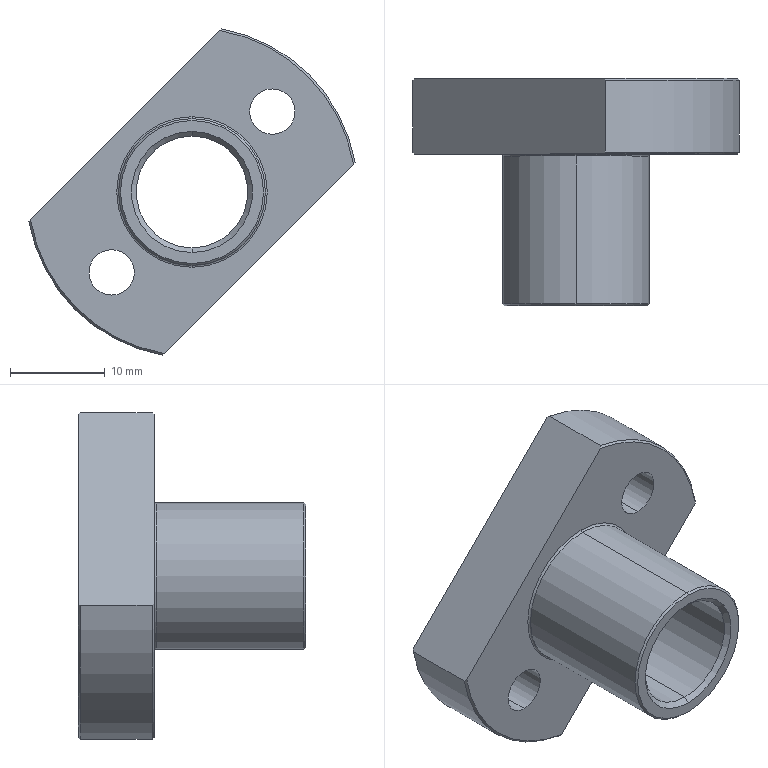Part | SolidWorks | features 3DProfileFeature 2, Chamfer 2, HoleWzd 2, Fillet 1, ICE 1, Revolution 1 | 1 solid | 33 faces | box 34.452 x 24 x 34.452 mm | volume 5075 mm3 | cylinder 14 | cone 10 | plane 7 | torus 2 | commonest cylinder face diameters 4.8 x4 8 x4 11.8 x2 15.5 x2 35 x2
STEP:
#1=CARTESIAN_POINT('',(0.,0.5,5.9));
#2=VERTEX_POINT('',#1);
#3=CARTESIAN_POINT('',(0.,0.5,-5.9));
#4=VERTEX_POINT('',#3);
#5=CARTESIAN_POINT('',(0.,0.5,0.));
#6=DIRECTION('',(0.,-1.,0.));
#7=DIRECTION('',(0.,0.,1.));
#8=AXIS2_PLACEMENT_3D('',#5,#6,#7);
#9=CIRCLE('',#8,5.9);
#10=EDGE_CURVE('',#2,#4,#9,.T.);
#11=ORIENTED_EDGE('',*,*,#10,.F.);
#12=CARTESIAN_POINT('',(0.,0.,6.4));
#13=VERTEX_POINT('',#12);
#14=CARTESIAN_POINT('',(0.,0.,6.4));
#15=DIRECTION('',(0.,-0.7071,0.7071));
#16=VECTOR('',#15,1000.);
#17=LINE('',#14,#16);
#18=EDGE_CURVE('',#2,#13,#17,.T.);
#19=ORIENTED_EDGE('',*,*,#18,.T.);
#20=CARTESIAN_POINT('',(0.,0.,-6.4));
#21=VERTEX_POINT('',#20);
#22=CARTESIAN_POINT('',(0.,0.,0.));
#23=DIRECTION('',(0.,1.,0.));
#24=DIRECTION('',(0.,0.,1.));
#25=AXIS2_PLACEMENT_3D('',#22,#23,#24);
#26=CIRCLE('',#25,6.4);
#27=EDGE_CURVE('',#21,#13,#26,.T.);
#28=ORIENTED_EDGE('',*,*,#27,.F.);
#29=CARTESIAN_POINT('',(0.,0.,-6.4));
#30=DIRECTION('',(0.,-0.7071,-0.7071));
#31=VECTOR('',#30,1000.);
#32=LINE('',#29,#31);
#33=EDGE_CURVE('',#4,#21,#32,.T.);
#34=ORIENTED_EDGE('',*,*,#33,.F.);
#35=EDGE_LOOP('',(#11,#19,#28,#34));
#36=FACE_OUTER_BOUND('',#35,.T.);
#37=CARTESIAN_POINT('',(0.,0.,0.));
#38=DIRECTION('',(0.,-1.,0.));
#39=DIRECTION('',(0.,0.,-1.));
#40=AXIS2_PLACEMENT_3D('',#37,#38,#39);
#41=CONICAL_SURFACE('',#40,6.4,0.7854);
#42=ADVANCED_FACE('',(#36),#41,.F.);
#43=CARTESIAN_POINT('',(0.,23.5,-5.9));
#44=VERTEX_POINT('',#43);
#45=CARTESIAN_POINT('',(0.,23.5,5.9));
#46=VERTEX_POINT('',#45);
#47=CARTESIAN_POINT('',(0.,23.5,0.));
#48=DIRECTION('',(0.,1.,0.));
#49=DIRECTION('',(0.,0.,-1.));
#50=AXIS2_PLACEMENT_3D('',#47,#48,#49);
#51=CIRCLE('',#50,5.9);
#52=EDGE_CURVE('',#44,#46,#51,.T.);
#53=ORIENTED_EDGE('',*,*,#52,.F.);
#54=CARTESIAN_POINT('',(0.,24.,-6.4));
#55=VERTEX_POINT('',#54);
#56=CARTESIAN_POINT('',(0.,23.5,-5.9));
#57=DIRECTION('',(0.,0.7071,-0.7071));
#58=VECTOR('',#57,1000.);
#59=LINE('',#56,#58);
#60=EDGE_CURVE('',#44,#55,#59,.T.);
#61=ORIENTED_EDGE('',*,*,#60,.T.);
#62=CARTESIAN_POINT('',(0.,24.,6.4));
#63=VERTEX_POINT('',#62);
#64=CARTESIAN_POINT('',(0.,24.,0.));
#65=DIRECTION('',(0.,-1.,0.));
#66=DIRECTION('',(0.,0.,-1.));
#67=AXIS2_PLACEMENT_3D('',#64,#65,#66);
#68=CIRCLE('',#67,6.4);
#69=EDGE_CURVE('',#63,#55,#68,.T.);
#70=ORIENTED_EDGE('',*,*,#69,.F.);
#71=CARTESIAN_POINT('',(0.,23.5,5.9));
#72=DIRECTION('',(0.,0.7071,0.7071));
#73=VECTOR('',#72,1000.);
#74=LINE('',#71,#73);
#75=EDGE_CURVE('',#46,#63,#74,.T.);
#76=ORIENTED_EDGE('',*,*,#75,.F.);
#77=EDGE_LOOP('',(#53,#61,#70,#76));
#78=FACE_OUTER_BOUND('',#77,.T.);
#79=CARTESIAN_POINT('',(0.,23.5,0.));
#80=DIRECTION('',(0.,1.,0.));
#81=DIRECTION('',(0.,0.,1.));
#82=AXIS2_PLACEMENT_3D('',#79,#80,#81);
#83=CONICAL_SURFACE('',#82,5.9,0.7854);
#84=ADVANCED_FACE('',(#78),#83,.F.);
#85=CARTESIAN_POINT('',(0.,0.,-7.55));
#86=VERTEX_POINT('',#85);
#87=CARTESIAN_POINT('',(0.,0.,7.55));
#88=VERTEX_POINT('',#87);
#89=CARTESIAN_POINT('',(0.,0.,0.));
#90=DIRECTION('',(0.,-1.,0.));
#91=DIRECTION('',(0.,0.,1.));
#92=AXIS2_PLACEMENT_3D('',#89,#90,#91);
#93=CIRCLE('',#92,7.55);
#94=EDGE_CURVE('',#86,#88,#93,.T.);
#95=ORIENTED_EDGE('',*,*,#94,.F.);
#96=CARTESIAN_POINT('',(0.,0.2,-7.75));
#97=VERTEX_POINT('',#96);
#98=CARTESIAN_POINT('',(0.,0.,-7.55));
#99=DIRECTION('',(0.,0.7071,-0.7071));
#100=VECTOR('',#99,1000.);
#101=LINE('',#98,#100);
#102=EDGE_CURVE('',#86,#97,#101,.T.);
#103=ORIENTED_EDGE('',*,*,#102,.T.);
#104=CARTESIAN_POINT('',(0.,0.2,7.75));
#105=VERTEX_POINT('',#104);
#106=CARTESIAN_POINT('',(0.,0.2,0.));
#107=DIRECTION('',(0.,1.,0.));
#108=DIRECTION('',(0.,0.,1.));
#109=AXIS2_PLACEMENT_3D('',#106,#107,#108);
#110=CIRCLE('',#109,7.75);
#111=EDGE_CURVE('',#105,#97,#110,.T.);
#112=ORIENTED_EDGE('',*,*,#111,.F.);
#113=CARTESIAN_POINT('',(0.,0.,7.55));
#114=DIRECTION('',(0.,0.7071,0.7071));
#115=VECTOR('',#114,1000.);
#116=LINE('',#113,#115);
#117=EDGE_CURVE('',#88,#105,#116,.T.);
#118=ORIENTED_EDGE('',*,*,#117,.F.);
#119=EDGE_LOOP('',(#95,#103,#112,#118));
#120=FACE_OUTER_BOUND('',#119,.T.);
#121=CARTESIAN_POINT('',(0.,0.,0.));
#122=DIRECTION('',(0.,1.,0.));
#123=DIRECTION('',(0.,0.,1.));
#124=AXIS2_PLACEMENT_3D('',#121,#122,#123);
#125=CONICAL_SURFACE('',#124,7.55,0.7854);
#126=ADVANCED_FACE('',(#120),#125,.T.);
#127=CARTESIAN_POINT('',(0.,16.,-7.95));
#128=VERTEX_POINT('',#127);
#129=CARTESIAN_POINT('',(0.,16.,7.95));
#130=VERTEX_POINT('',#129);
#131=CARTESIAN_POINT('',(0.,16.,0.));
#132=DIRECTION('',(0.,1.,0.));
#133=DIRECTION('',(0.,0.,1.));
#134=AXIS2_PLACEMENT_3D('',#131,#132,#133);
#135=CIRCLE('',#134,7.95);
#136=EDGE_CURVE('',#128,#130,#135,.T.);
#137=ORIENTED_EDGE('',*,*,#136,.F.);
#138=CARTESIAN_POINT('',(0.,15.8,-7.75));
#139=VERTEX_POINT('',#138);
#140=CARTESIAN_POINT('',(0.,15.8,-7.95));
#141=DIRECTION('',(1.,0.,0.));
#142=DIRECTION('',(0.,0.,-1.));
#143=AXIS2_PLACEMENT_3D('',#140,#141,#142);
#144=CIRCLE('',#143,0.2);
#145=EDGE_CURVE('',#128,#139,#144,.T.);
#146=ORIENTED_EDGE('',*,*,#145,.T.);
#147=CARTESIAN_POINT('',(0.,15.8,7.75));
#148=VERTEX_POINT('',#147);
#149=CARTESIAN_POINT('',(0.,15.8,0.));
#150=DIRECTION('',(0.,-1.,0.));
#151=DIRECTION('',(0.,0.,1.));
#152=AXIS2_PLACEMENT_3D('',#149,#150,#151);
#153=CIRCLE('',#152,7.75);
#154=EDGE_CURVE('',#148,#139,#153,.T.);
#155=ORIENTED_EDGE('',*,*,#154,.F.);
#156=CARTESIAN_POINT('',(0.,15.8,7.95));
#157=DIRECTION('',(-1.,0.,0.));
#158=DIRECTION('',(0.,-1.,0.));
#159=AXIS2_PLACEMENT_3D('',#156,#157,#158);
#160=CIRCLE('',#159,0.2);
#161=EDGE_CURVE('',#130,#148,#160,.T.);
#162=ORIENTED_EDGE('',*,*,#161,.F.);
#163=EDGE_LOOP('',(#137,#146,#155,#162));
#164=FACE_OUTER_BOUND('',#163,.T.);
#165=CARTESIAN_POINT('',(0.,15.8,0.));
#166=DIRECTION('',(0.,1.,0.));
#167=DIRECTION('',(0.,0.,1.));
#168=AXIS2_PLACEMENT_3D('',#165,#166,#167);
#169=TOROIDAL_SURFACE('',#168,7.95,0.2);
#170=ADVANCED_FACE('',(#164),#169,.F.);
#171=CARTESIAN_POINT('',(-8.485,19.4,-12.485));
#172=VERTEX_POINT('',#171);
#173=CARTESIAN_POINT('',(-8.485,19.4,-4.485));
#174=VERTEX_POINT('',#173);
#175=CARTESIAN_POINT('',(-8.485,19.4,-8.485));
#176=DIRECTION('',(0.,1.,0.));
#177=DIRECTION('',(0.,0.,1.));
#178=AXIS2_PLACEMENT_3D('',#175,#176,#177);
#179=CIRCLE('',#178,4.);
#180=EDGE_CURVE('',#172,#174,#179,.T.);
#181=ORIENTED_EDGE('',*,*,#180,.F.);
#182=CARTESIAN_POINT('',(-8.485,24.,-12.485));
#183=VERTEX_POINT('',#182);
#184=CARTESIAN_POINT('',(-8.485,24.,-12.485));
#185=DIRECTION('',(0.,1.,0.));
#186=VECTOR('',#185,1000.);
#187=LINE('',#184,#186);
#188=EDGE_CURVE('',#172,#183,#187,.T.);
#189=ORIENTED_EDGE('',*,*,#188,.T.);
#190=CARTESIAN_POINT('',(-8.485,24.,-4.485));
#191=VERTEX_POINT('',#190);
#192=CARTESIAN_POINT('',(-8.485,24.,-8.485));
#193=DIRECTION('',(0.,1.,0.));
#194=DIRECTION('',(0.,0.,1.));
#195=AXIS2_PLACEMENT_3D('',#192,#193,#194);
#196=CIRCLE('',#195,4.);
#197=EDGE_CURVE('',#183,#191,#196,.T.);
#198=ORIENTED_EDGE('',*,*,#197,.T.);
#199=CARTESIAN_POINT('',(-8.485,24.,-4.485));
#200=DIRECTION('',(0.,1.,0.));
#201=VECTOR('',#200,1000.);
#202=LINE('',#199,#201);
#203=EDGE_CURVE('',#174,#191,#202,.T.);
#204=ORIENTED_EDGE('',*,*,#203,.F.);
#205=EDGE_LOOP('',(#181,#189,#198,#204));
#206=FACE_OUTER_BOUND('',#205,.T.);
#207=CARTESIAN_POINT('',(-8.485,24.,-8.485));
#208=DIRECTION('',(0.,1.,0.));
#209=DIRECTION('',(0.,0.,1.));
#210=AXIS2_PLACEMENT_3D('',#207,#208,#209);
#211=CYLINDRICAL_SURFACE('',#210,4.);
#212=ADVANCED_FACE('',(#206),#211,.F.);
#213=CARTESIAN_POINT('',(-8.485,16.,-10.885));
#214=VERTEX_POINT('',#213);
#215=CARTESIAN_POINT('',(-8.485,16.,-6.085));
#216=VERTEX_POINT('',#215);
#217=CARTESIAN_POINT('',(-8.485,16.,-8.485));
#218=DIRECTION('',(0.,1.,0.));
#219=DIRECTION('',(0.,0.,1.));
#220=AXIS2_PLACEMENT_3D('',#217,#218,#219);
#221=CIRCLE('',#220,2.4);
#222=EDGE_CURVE('',#214,#216,#221,.T.);
#223=ORIENTED_EDGE('',*,*,#222,.F.);
#224=CARTESIAN_POINT('',(-8.485,19.4,-10.885));
#225=VERTEX_POINT('',#224);
#226=CARTESIAN_POINT('',(-8.485,24.,-10.885));
#227=DIRECTION('',(0.,1.,0.));
#228=VECTOR('',#227,1000.);
#229=LINE('',#226,#228);
#230=EDGE_CURVE('',#214,#225,#229,.T.);
#231=ORIENTED_EDGE('',*,*,#230,.T.);
#232=CARTESIAN_POINT('',(-8.485,19.4,-6.085));
#233=VERTEX_POINT('',#232);
#234=CARTESIAN_POINT('',(-8.485,19.4,-8.485));
#235=DIRECTION('',(0.,1.,0.));
#236=DIRECTION('',(0.,0.,1.));
#237=AXIS2_PLACEMENT_3D('',#234,#235,#236);
#238=CIRCLE('',#237,2.4);
#239=EDGE_CURVE('',#225,#233,#238,.T.);
#240=ORIENTED_EDGE('',*,*,#239,.T.);
#241=CARTESIAN_POINT('',(-8.485,24.,-6.085));
#242=DIRECTION('',(0.,1.,0.));
#243=VECTOR('',#242,1000.);
#244=LINE('',#241,#243);
#245=EDGE_CURVE('',#216,#233,#244,.T.);
#246=ORIENTED_EDGE('',*,*,#245,.F.);
#247=EDGE_LOOP('',(#223,#231,#240,#246));
#248=FACE_OUTER_BOUND('',#247,.T.);
#249=CARTESIAN_POINT('',(-8.485,24.,-8.485));
#250=DIRECTION('',(0.,1.,0.));
#251=DIRECTION('',(0.,0.,1.));
#252=AXIS2_PLACEMENT_3D('',#249,#250,#251);
#253=CYLINDRICAL_SURFACE('',#252,2.4);
#254=ADVANCED_FACE('',(#248),#253,.F.);
#255=CARTESIAN_POINT('',(8.485,19.4,4.485));
#256=VERTEX_POINT('',#255);
#257=CARTESIAN_POINT('',(8.485,19.4,12.485));
#258=VERTEX_POINT('',#257);
#259=CARTESIAN_POINT('',(8.485,19.4,8.485));
#260=DIRECTION('',(0.,1.,0.));
#261=DIRECTION('',(0.,0.,1.));
#262=AXIS2_PLACEMENT_3D('',#259,#260,#261);
#263=CIRCLE('',#262,4.);
#264=EDGE_CURVE('',#256,#258,#263,.T.);
#265=ORIENTED_EDGE('',*,*,#264,.F.);
#266=CARTESIAN_POINT('',(8.485,24.,4.485));
#267=VERTEX_POINT('',#266);
#268=CARTESIAN_POINT('',(8.485,24.,4.485));
#269=DIRECTION('',(0.,1.,0.));
#270=VECTOR('',#269,1000.);
#271=LINE('',#268,#270);
#272=EDGE_CURVE('',#256,#267,#271,.T.);
#273=ORIENTED_EDGE('',*,*,#272,.T.);
#274=CARTESIAN_POINT('',(8.485,24.,12.485));
#275=VERTEX_POINT('',#274);
#276=CARTESIAN_POINT('',(8.485,24.,8.485));
#277=DIRECTION('',(0.,1.,0.));
#278=DIRECTION('',(0.,0.,1.));
#279=AXIS2_PLACEMENT_3D('',#276,#277,#278);
#280=CIRCLE('',#279,4.);
#281=EDGE_CURVE('',#267,#275,#280,.T.);
#282=ORIENTED_EDGE('',*,*,#281,.T.);
#283=CARTESIAN_POINT('',(8.485,24.,12.485));
#284=DIRECTION('',(0.,1.,0.));
#285=VECTOR('',#284,1000.);
#286=LINE('',#283,#285);
#287=EDGE_CURVE('',#258,#275,#286,.T.);
#288=ORIENTED_EDGE('',*,*,#287,.F.);
#289=EDGE_LOOP('',(#265,#273,#282,#288));
#290=FACE_OUTER_BOUND('',#289,.T.);
#291=CARTESIAN_POINT('',(8.485,24.,8.485));
#292=DIRECTION('',(0.,1.,0.));
#293=DIRECTION('',(0.,0.,1.));
#294=AXIS2_PLACEMENT_3D('',#291,#292,#293);
#295=CYLINDRICAL_SURFACE('',#294,4.);
#296=ADVANCED_FACE('',(#290),#295,.F.);
#297=CARTESIAN_POINT('',(8.485,16.,6.085));
#298=VERTEX_POINT('',#297);
#299=CARTESIAN_POINT('',(8.485,16.,10.885));
#300=VERTEX_POINT('',#299);
#301=CARTESIAN_POINT('',(8.485,16.,8.485));
#302=DIRECTION('',(0.,1.,0.));
#303=DIRECTION('',(0.,0.,1.));
#304=AXIS2_PLACEMENT_3D('',#301,#302,#303);
#305=CIRCLE('',#304,2.4);
#306=EDGE_CURVE('',#298,#300,#305,.T.);
#307=ORIENTED_EDGE('',*,*,#306,.F.);
#308=CARTESIAN_POINT('',(8.485,19.4,6.085));
#309=VERTEX_POINT('',#308);
#310=CARTESIAN_POINT('',(8.485,24.,6.085));
#311=DIRECTION('',(0.,1.,0.));
#312=VECTOR('',#311,1000.);
#313=LINE('',#310,#312);
#314=EDGE_CURVE('',#298,#309,#313,.T.);
#315=ORIENTED_EDGE('',*,*,#314,.T.);
#316=CARTESIAN_POINT('',(8.485,19.4,10.885));
#317=VERTEX_POINT('',#316);
#318=CARTESIAN_POINT('',(8.485,19.4,8.485));
#319=DIRECTION('',(0.,1.,0.));
#320=DIRECTION('',(0.,0.,1.));
#321=AXIS2_PLACEMENT_3D('',#318,#319,#320);
#322=CIRCLE('',#321,2.4);
#323=EDGE_CURVE('',#309,#317,#322,.T.);
#324=ORIENTED_EDGE('',*,*,#323,.T.);
#325=CARTESIAN_POINT('',(8.485,24.,10.885));
#326=DIRECTION('',(0.,1.,0.));
#327=VECTOR('',#326,1000.);
#328=LINE('',#325,#327);
#329=EDGE_CURVE('',#300,#317,#328,.T.);
#330=ORIENTED_EDGE('',*,*,#329,.F.);
#331=EDGE_LOOP('',(#307,#315,#324,#330));
#332=FACE_OUTER_BOUND('',#331,.T.);
#333=CARTESIAN_POINT('',(8.485,24.,8.485));
#334=DIRECTION('',(0.,1.,0.));
#335=DIRECTION('',(0.,0.,1.));
#336=AXIS2_PLACEMENT_3D('',#333,#334,#335);
#337=CYLINDRICAL_SURFACE('',#336,2.4);
#338=ADVANCED_FACE('',(#332),#337,.F.);
#339=ORIENTED_EDGE('',*,*,#10,.T.);
#340=CARTESIAN_POINT('',(0.,24.,-5.9));
#341=DIRECTION('',(0.,1.,0.));
#342=VECTOR('',#341,1000.);
#343=LINE('',#340,#342);
#344=EDGE_CURVE('',#4,#44,#343,.T.);
#345=ORIENTED_EDGE('',*,*,#344,.T.);
#346=ORIENTED_EDGE('',*,*,#52,.T.);
#347=CARTESIAN_POINT('',(0.,24.,5.9));
#348=DIRECTION('',(0.,1.,0.));
#349=VECTOR('',#348,1000.);
#350=LINE('',#347,#349);
#351=EDGE_CURVE('',#2,#46,#350,.T.);
#352=ORIENTED_EDGE('',*,*,#351,.F.);
#353=EDGE_LOOP('',(#339,#345,#346,#352));
#354=FACE_OUTER_BOUND('',#353,.T.);
#355=CARTESIAN_POINT('',(0.,24.,0.));
#356=DIRECTION('',(0.,1.,0.));
#357=DIRECTION('',(0.,0.,1.));
#358=AXIS2_PLACEMENT_3D('',#355,#356,#357);
#359=CYLINDRICAL_SURFACE('',#358,5.9);
#360=ADVANCED_FACE('',(#354),#359,.F.);
#361=CARTESIAN_POINT('',(0.,15.8,0.));
#362=DIRECTION('',(0.,-1.,0.));
#363=DIRECTION('',(0.,0.,1.));
#364=AXIS2_PLACEMENT_3D('',#361,#362,#363);
#365=CIRCLE('',#364,7.75);
#366=EDGE_CURVE('',#139,#148,#365,.T.);
#367=ORIENTED_EDGE('',*,*,#366,.T.);
#368=CARTESIAN_POINT('',(0.,0.,7.75));
#369=DIRECTION('',(0.,-1.,0.));
#370=VECTOR('',#369,1000.);
#371=LINE('',#368,#370);
#372=EDGE_CURVE('',#148,#105,#371,.T.);
#373=ORIENTED_EDGE('',*,*,#372,.T.);
#374=ORIENTED_EDGE('',*,*,#111,.T.);
#375=CARTESIAN_POINT('',(0.,0.,-7.75));
#376=DIRECTION('',(0.,-1.,0.));
#377=VECTOR('',#376,1000.);
#378=LINE('',#375,#377);
#379=EDGE_CURVE('',#139,#97,#378,.T.);
#380=ORIENTED_EDGE('',*,*,#379,.F.);
#381=EDGE_LOOP('',(#367,#373,#374,#380));
#382=FACE_OUTER_BOUND('',#381,.T.);
#383=CARTESIAN_POINT('',(0.,0.,0.));
#384=DIRECTION('',(0.,-1.,0.));
#385=DIRECTION('',(0.,0.,-1.));
#386=AXIS2_PLACEMENT_3D('',#383,#384,#385);
#387=CYLINDRICAL_SURFACE('',#386,7.75);
#388=ADVANCED_FACE('',(#382),#387,.T.);
#389=CARTESIAN_POINT('',(-8.485,24.,-8.485));
#390=DIRECTION('',(0.,1.,0.));
#391=DIRECTION('',(0.,0.,1.));
#392=AXIS2_PLACEMENT_3D('',#389,#390,#391);
#393=CIRCLE('',#392,4.);
#394=EDGE_CURVE('',#191,#183,#393,.T.);
#395=ORIENTED_EDGE('',*,*,#394,.F.);
#396=ORIENTED_EDGE('',*,*,#197,.F.);
#397=EDGE_LOOP('',(#395,#396));
#398=FACE_BOUND('',#397,.T.);
#399=CARTESIAN_POINT('',(8.485,24.,8.485));
#400=DIRECTION('',(0.,1.,0.));
#401=DIRECTION('',(0.,0.,1.));
#402=AXIS2_PLACEMENT_3D('',#399,#400,#401);
#403=CIRCLE('',#402,4.);
#404=EDGE_CURVE('',#275,#267,#403,.T.);
#405=ORIENTED_EDGE('',*,*,#404,.F.);
#406=ORIENTED_EDGE('',*,*,#281,.F.);
#407=EDGE_LOOP('',(#405,#406));
#408=FACE_BOUND('',#407,.T.);
#409=ORIENTED_EDGE('',*,*,#69,.T.);
#410=CARTESIAN_POINT('',(0.,24.,0.));
#411=DIRECTION('',(0.,-1.,0.));
#412=DIRECTION('',(0.,0.,-1.));
#413=AXIS2_PLACEMENT_3D('',#410,#411,#412);
#414=CIRCLE('',#413,6.4);
#415=EDGE_CURVE('',#55,#63,#414,.T.);
#416=ORIENTED_EDGE('',*,*,#415,.T.);
#417=EDGE_LOOP('',(#409,#416));
#418=FACE_BOUND('',#417,.T.);
#419=CARTESIAN_POINT('',(2.911,24.,17.053));
#420=VERTEX_POINT('',#419);
#421=CARTESIAN_POINT('',(17.053,24.,2.911));
#422=VERTEX_POINT('',#421);
#423=CARTESIAN_POINT('',(0.,24.,0.));
#424=DIRECTION('',(0.,1.,0.));
#425=DIRECTION('',(0.,0.,-1.));
#426=AXIS2_PLACEMENT_3D('',#423,#424,#425);
#427=CIRCLE('',#426,17.3);
#428=EDGE_CURVE('',#420,#422,#427,.T.);
#429=ORIENTED_EDGE('',*,*,#428,.T.);
#430=CARTESIAN_POINT('',(-2.911,24.,-17.053));
#431=VERTEX_POINT('',#430);
#432=CARTESIAN_POINT('',(7.071,24.,-7.071));
#433=DIRECTION('',(0.7071,0.,0.7071));
#434=VECTOR('',#433,1000.);
#435=LINE('',#432,#434);
#436=EDGE_CURVE('',#431,#422,#435,.T.);
#437=ORIENTED_EDGE('',*,*,#436,.F.);
#438=CARTESIAN_POINT('',(-17.053,24.,-2.911));
#439=VERTEX_POINT('',#438);
#440=CARTESIAN_POINT('',(0.,24.,0.));
#441=DIRECTION('',(0.,1.,0.));
#442=DIRECTION('',(0.,0.,-1.));
#443=AXIS2_PLACEMENT_3D('',#440,#441,#442);
#444=CIRCLE('',#443,17.3);
#445=EDGE_CURVE('',#431,#439,#444,.T.);
#446=ORIENTED_EDGE('',*,*,#445,.T.);
#447=CARTESIAN_POINT('',(-7.071,24.,7.071));
#448=DIRECTION('',(0.7071,0.,0.7071));
#449=VECTOR('',#448,1000.);
#450=LINE('',#447,#449);
#451=EDGE_CURVE('',#439,#420,#450,.T.);
#452=ORIENTED_EDGE('',*,*,#451,.T.);
#453=EDGE_LOOP('',(#429,#437,#446,#452));
#454=FACE_OUTER_BOUND('',#453,.T.);
#455=CARTESIAN_POINT('',(0.,24.,0.));
#456=DIRECTION('',(0.,-1.,0.));
#457=DIRECTION('',(0.,0.,-1.));
#458=AXIS2_PLACEMENT_3D('',#455,#456,#457);
#459=PLANE('',#458);
#460=ADVANCED_FACE('',(#398,#408,#418,#454),#459,.F.);
#461=CARTESIAN_POINT('',(-17.226,23.8,-3.084));
#462=VERTEX_POINT('',#461);
#463=CARTESIAN_POINT('',(-3.084,23.8,-17.226));
#464=VERTEX_POINT('',#463);
#465=CARTESIAN_POINT('',(0.,23.8,0.));
#466=DIRECTION('',(0.,-1.,0.));
#467=DIRECTION('',(0.,0.,-1.));
#468=AXIS2_PLACEMENT_3D('',#465,#466,#467);
#469=CIRCLE('',#468,17.5);
#470=EDGE_CURVE('',#462,#464,#469,.T.);
#471=ORIENTED_EDGE('',*,*,#470,.T.);
#472=CARTESIAN_POINT('',(-3.084,16.2,-17.226));
#473=VERTEX_POINT('',#472);
#474=CARTESIAN_POINT('',(-3.084,0.,-17.226));
#475=DIRECTION('',(0.,1.,0.));
#476=VECTOR('',#475,1000.);
#477=LINE('',#474,#476);
#478=EDGE_CURVE('',#473,#464,#477,.T.);
#479=ORIENTED_EDGE('',*,*,#478,.F.);
#480=CARTESIAN_POINT('',(-17.226,16.2,-3.084));
#481=VERTEX_POINT('',#480);
#482=CARTESIAN_POINT('',(0.,16.2,0.));
#483=DIRECTION('',(0.,1.,0.));
#484=DIRECTION('',(0.,0.,1.));
#485=AXIS2_PLACEMENT_3D('',#482,#483,#484);
#486=CIRCLE('',#485,17.5);
#487=EDGE_CURVE('',#473,#481,#486,.T.);
#488=ORIENTED_EDGE('',*,*,#487,.T.);
#489=CARTESIAN_POINT('',(-17.226,0.,-3.084));
#490=DIRECTION('',(0.,1.,0.));
#491=VECTOR('',#490,1000.);
#492=LINE('',#489,#491);
#493=EDGE_CURVE('',#481,#462,#492,.T.);
#494=ORIENTED_EDGE('',*,*,#493,.T.);
#495=EDGE_LOOP('',(#471,#479,#488,#494));
#496=FACE_OUTER_BOUND('',#495,.T.);
#497=CARTESIAN_POINT('',(0.,0.,0.));
#498=DIRECTION('',(0.,-1.,0.));
#499=DIRECTION('',(0.,0.,-1.));
#500=AXIS2_PLACEMENT_3D('',#497,#498,#499);
#501=CYLINDRICAL_SURFACE('',#500,17.5);
#502=ADVANCED_FACE('',(#496),#501,.T.);
#503=CARTESIAN_POINT('',(3.084,16.2,17.226));
#504=VERTEX_POINT('',#503);
#505=CARTESIAN_POINT('',(17.226,16.2,3.084));
#506=VERTEX_POINT('',#505);
#507=CARTESIAN_POINT('',(0.,16.2,0.));
#508=DIRECTION('',(0.,1.,0.));
#509=DIRECTION('',(0.,0.,1.));
#510=AXIS2_PLACEMENT_3D('',#507,#508,#509);
#511=CIRCLE('',#510,17.5);
#512=EDGE_CURVE('',#504,#506,#511,.T.);
#513=ORIENTED_EDGE('',*,*,#512,.T.);
#514=CARTESIAN_POINT('',(17.226,23.8,3.084));
#515=VERTEX_POINT('',#514);
#516=CARTESIAN_POINT('',(17.226,0.,3.084));
#517=DIRECTION('',(0.,1.,0.));
#518=VECTOR('',#517,1000.);
#519=LINE('',#516,#518);
#520=EDGE_CURVE('',#506,#515,#519,.T.);
#521=ORIENTED_EDGE('',*,*,#520,.T.);
#522=CARTESIAN_POINT('',(3.084,23.8,17.226));
#523=VERTEX_POINT('',#522);
#524=CARTESIAN_POINT('',(0.,23.8,0.));
#525=DIRECTION('',(0.,-1.,0.));
#526=DIRECTION('',(0.,0.,-1.));
#527=AXIS2_PLACEMENT_3D('',#524,#525,#526);
#528=CIRCLE('',#527,17.5);
#529=EDGE_CURVE('',#515,#523,#528,.T.);
#530=ORIENTED_EDGE('',*,*,#529,.T.);
#531=CARTESIAN_POINT('',(3.084,0.,17.226));
#532=DIRECTION('',(0.,1.,0.));
#533=VECTOR('',#532,1000.);
#534=LINE('',#531,#533);
#535=EDGE_CURVE('',#504,#523,#534,.T.);
#536=ORIENTED_EDGE('',*,*,#535,.F.);
#537=EDGE_LOOP('',(#513,#521,#530,#536));
#538=FACE_OUTER_BOUND('',#537,.T.);
#539=CARTESIAN_POINT('',(0.,0.,0.));
#540=DIRECTION('',(0.,-1.,0.));
#541=DIRECTION('',(0.,0.,-1.));
#542=AXIS2_PLACEMENT_3D('',#539,#540,#541);
#543=CYLINDRICAL_SURFACE('',#542,17.5);
#544=ADVANCED_FACE('',(#538),#543,.T.);
#545=CARTESIAN_POINT('',(8.485,16.,8.485));
#546=DIRECTION('',(0.,1.,0.));
#547=DIRECTION('',(0.,0.,1.));
#548=AXIS2_PLACEMENT_3D('',#545,#546,#547);
#549=CIRCLE('',#548,2.4);
#550=EDGE_CURVE('',#300,#298,#549,.T.);
#551=ORIENTED_EDGE('',*,*,#550,.T.);
#552=ORIENTED_EDGE('',*,*,#306,.T.);
#553=EDGE_LOOP('',(#551,#552));
#554=FACE_BOUND('',#553,.T.);
#555=CARTESIAN_POINT('',(-8.485,16.,-8.485));
#556=DIRECTION('',(0.,1.,0.));
#557=DIRECTION('',(0.,0.,1.));
#558=AXIS2_PLACEMENT_3D('',#555,#556,#557);
#559=CIRCLE('',#558,2.4);
#560=EDGE_CURVE('',#216,#214,#559,.T.);
#561=ORIENTED_EDGE('',*,*,#560,.T.);
#562=ORIENTED_EDGE('',*,*,#222,.T.);
#563=EDGE_LOOP('',(#561,#562));
#564=FACE_BOUND('',#563,.T.);
#565=CARTESIAN_POINT('',(0.,16.,0.));
#566=DIRECTION('',(0.,1.,0.));
#567=DIRECTION('',(0.,0.,1.));
#568=AXIS2_PLACEMENT_3D('',#565,#566,#567);
#569=CIRCLE('',#568,7.95);
#570=EDGE_CURVE('',#130,#128,#569,.T.);
#571=ORIENTED_EDGE('',*,*,#570,.T.);
#572=ORIENTED_EDGE('',*,*,#136,.T.);
#573=EDGE_LOOP('',(#571,#572));
#574=FACE_BOUND('',#573,.T.);
#575=CARTESIAN_POINT('',(-17.053,16.,-2.911));
#576=VERTEX_POINT('',#575);
#577=CARTESIAN_POINT('',(-2.911,16.,-17.053));
#578=VERTEX_POINT('',#577);
#579=CARTESIAN_POINT('',(0.,16.,0.));
#580=DIRECTION('',(0.,-1.,0.));
#581=DIRECTION('',(0.,0.,1.));
#582=AXIS2_PLACEMENT_3D('',#579,#580,#581);
#583=CIRCLE('',#582,17.3);
#584=EDGE_CURVE('',#576,#578,#583,.T.);
#585=ORIENTED_EDGE('',*,*,#584,.T.);
#586=CARTESIAN_POINT('',(17.053,16.,2.911));
#587=VERTEX_POINT('',#586);
#588=CARTESIAN_POINT('',(-1.679,16.,-15.821));
#589=DIRECTION('',(0.7071,0.,0.7071));
#590=VECTOR('',#589,1000.);
#591=LINE('',#588,#590);
#592=EDGE_CURVE('',#578,#587,#591,.T.);
#593=ORIENTED_EDGE('',*,*,#592,.T.);
#594=CARTESIAN_POINT('',(2.911,16.,17.053));
#595=VERTEX_POINT('',#594);
#596=CARTESIAN_POINT('',(0.,16.,0.));
#597=DIRECTION('',(0.,-1.,0.));
#598=DIRECTION('',(0.,0.,1.));
#599=AXIS2_PLACEMENT_3D('',#596,#597,#598);
#600=CIRCLE('',#599,17.3);
#601=EDGE_CURVE('',#587,#595,#600,.T.);
#602=ORIENTED_EDGE('',*,*,#601,.T.);
#603=CARTESIAN_POINT('',(-15.821,16.,-1.679));
#604=DIRECTION('',(0.7071,0.,0.7071));
#605=VECTOR('',#604,1000.);
#606=LINE('',#603,#605);
#607=EDGE_CURVE('',#576,#595,#606,.T.);
#608=ORIENTED_EDGE('',*,*,#607,.F.);
#609=EDGE_LOOP('',(#585,#593,#602,#608));
#610=FACE_OUTER_BOUND('',#609,.T.);
#611=CARTESIAN_POINT('',(-17.5,16.,0.));
#612=DIRECTION('',(0.,1.,0.));
#613=DIRECTION('',(0.,0.,1.));
#614=AXIS2_PLACEMENT_3D('',#611,#612,#613);
#615=PLANE('',#614);
#616=ADVANCED_FACE('',(#554,#564,#574,#610),#615,.F.);
#617=CARTESIAN_POINT('',(-3.084,23.8,-17.226));
#618=CARTESIAN_POINT('',(-3.026,23.867,-17.169));
#619=CARTESIAN_POINT('',(-2.969,23.933,-17.111));
#620=CARTESIAN_POINT('',(-2.911,24.,-17.053));
#621=B_SPLINE_CURVE_WITH_KNOTS('',3,(#617,#618,#619,#620),.UNSPECIFIED.,.F.,.F.,(4,4),(0.02558,0.0259),.UNSPECIFIED.);
#622=EDGE_CURVE('',#464,#431,#621,.T.);
#623=ORIENTED_EDGE('',*,*,#622,.F.);
#624=ORIENTED_EDGE('',*,*,#470,.F.);
#625=CARTESIAN_POINT('',(-17.226,23.8,-3.084));
#626=CARTESIAN_POINT('',(-17.169,23.867,-3.026));
#627=CARTESIAN_POINT('',(-17.111,23.933,-2.969));
#628=CARTESIAN_POINT('',(-17.053,24.,-2.911));
#629=B_SPLINE_CURVE_WITH_KNOTS('',3,(#625,#626,#627,#628),.UNSPECIFIED.,.F.,.F.,(4,4),(0.02558,0.0259),.UNSPECIFIED.);
#630=EDGE_CURVE('',#462,#439,#629,.T.);
#631=ORIENTED_EDGE('',*,*,#630,.T.);
#632=ORIENTED_EDGE('',*,*,#445,.F.);
#633=EDGE_LOOP('',(#623,#624,#631,#632));
#634=FACE_OUTER_BOUND('',#633,.T.);
#635=CARTESIAN_POINT('',(0.,23.8,0.));
#636=DIRECTION('',(0.,-1.,0.));
#637=DIRECTION('',(0.,0.,-1.));
#638=AXIS2_PLACEMENT_3D('',#635,#636,#637);
#639=CONICAL_SURFACE('',#638,17.5,0.7854);
#640=ADVANCED_FACE('',(#634),#639,.T.);
#641=CARTESIAN_POINT('',(17.053,24.,2.911));
#642=CARTESIAN_POINT('',(17.111,23.933,2.969));
#643=CARTESIAN_POINT('',(17.169,23.867,3.026));
#644=CARTESIAN_POINT('',(17.226,23.8,3.084));
#645=B_SPLINE_CURVE_WITH_KNOTS('',3,(#641,#642,#643,#644),.UNSPECIFIED.,.F.,.F.,(4,4),(0.05834,0.05866),.UNSPECIFIED.);
#646=EDGE_CURVE('',#422,#515,#645,.T.);
#647=ORIENTED_EDGE('',*,*,#646,.F.);
#648=ORIENTED_EDGE('',*,*,#428,.F.);
#649=CARTESIAN_POINT('',(2.911,24.,17.053));
#650=CARTESIAN_POINT('',(2.969,23.933,17.111));
#651=CARTESIAN_POINT('',(3.026,23.867,17.169));
#652=CARTESIAN_POINT('',(3.084,23.8,17.226));
#653=B_SPLINE_CURVE_WITH_KNOTS('',3,(#649,#650,#651,#652),.UNSPECIFIED.,.F.,.F.,(4,4),(0.05834,0.05866),.UNSPECIFIED.);
#654=EDGE_CURVE('',#420,#523,#653,.T.);
#655=ORIENTED_EDGE('',*,*,#654,.T.);
#656=ORIENTED_EDGE('',*,*,#529,.F.);
#657=EDGE_LOOP('',(#647,#648,#655,#656));
#658=FACE_OUTER_BOUND('',#657,.T.);
#659=CARTESIAN_POINT('',(0.,23.8,0.));
#660=DIRECTION('',(0.,-1.,0.));
#661=DIRECTION('',(0.,0.,-1.));
#662=AXIS2_PLACEMENT_3D('',#659,#660,#661);
#663=CONICAL_SURFACE('',#662,17.5,0.7854);
#664=ADVANCED_FACE('',(#658),#663,.T.);
#665=CARTESIAN_POINT('',(17.226,16.2,3.084));
#666=CARTESIAN_POINT('',(17.169,16.133,3.026));
#667=CARTESIAN_POINT('',(17.111,16.067,2.969));
#668=CARTESIAN_POINT('',(17.053,16.,2.911));
#669=B_SPLINE_CURVE_WITH_KNOTS('',3,(#665,#666,#667,#668),.UNSPECIFIED.,.F.,.F.,(4,4),(0.02558,0.0259),.UNSPECIFIED.);
#670=EDGE_CURVE('',#506,#587,#669,.T.);
#671=ORIENTED_EDGE('',*,*,#670,.F.);
#672=ORIENTED_EDGE('',*,*,#512,.F.);
#673=CARTESIAN_POINT('',(3.084,16.2,17.226));
#674=CARTESIAN_POINT('',(3.026,16.133,17.169));
#675=CARTESIAN_POINT('',(2.969,16.067,17.111));
#676=CARTESIAN_POINT('',(2.911,16.,17.053));
#677=B_SPLINE_CURVE_WITH_KNOTS('',3,(#673,#674,#675,#676),.UNSPECIFIED.,.F.,.F.,(4,4),(0.02558,0.0259),.UNSPECIFIED.);
#678=EDGE_CURVE('',#504,#595,#677,.T.);
#679=ORIENTED_EDGE('',*,*,#678,.T.);
#680=ORIENTED_EDGE('',*,*,#601,.F.);
#681=EDGE_LOOP('',(#671,#672,#679,#680));
#682=FACE_OUTER_BOUND('',#681,.T.);
#683=CARTESIAN_POINT('',(0.,16.,0.));
#684=DIRECTION('',(0.,1.,0.));
#685=DIRECTION('',(0.,0.,1.));
#686=AXIS2_PLACEMENT_3D('',#683,#684,#685);
#687=CONICAL_SURFACE('',#686,17.3,0.7854);
#688=ADVANCED_FACE('',(#682),#687,.T.);
#689=CARTESIAN_POINT('',(-2.911,16.,-17.053));
#690=CARTESIAN_POINT('',(-2.969,16.067,-17.111));
#691=CARTESIAN_POINT('',(-3.026,16.133,-17.169));
#692=CARTESIAN_POINT('',(-3.084,16.2,-17.226));
#693=B_SPLINE_CURVE_WITH_KNOTS('',3,(#689,#690,#691,#692),.UNSPECIFIED.,.F.,.F.,(4,4),(0.05834,0.05866),.UNSPECIFIED.);
#694=EDGE_CURVE('',#578,#473,#693,.T.);
#695=ORIENTED_EDGE('',*,*,#694,.F.);
#696=ORIENTED_EDGE('',*,*,#584,.F.);
#697=CARTESIAN_POINT('',(-17.053,16.,-2.911));
#698=CARTESIAN_POINT('',(-17.111,16.067,-2.969));
#699=CARTESIAN_POINT('',(-17.169,16.133,-3.026));
#700=CARTESIAN_POINT('',(-17.226,16.2,-3.084));
#701=B_SPLINE_CURVE_WITH_KNOTS('',3,(#697,#698,#699,#700),.UNSPECIFIED.,.F.,.F.,(4,4),(0.05834,0.05866),.UNSPECIFIED.);
#702=EDGE_CURVE('',#576,#481,#701,.T.);
#703=ORIENTED_EDGE('',*,*,#702,.T.);
#704=ORIENTED_EDGE('',*,*,#487,.F.);
#705=EDGE_LOOP('',(#695,#696,#703,#704));
#706=FACE_OUTER_BOUND('',#705,.T.);
#707=CARTESIAN_POINT('',(0.,16.,0.));
#708=DIRECTION('',(0.,1.,0.));
#709=DIRECTION('',(0.,0.,1.));
#710=AXIS2_PLACEMENT_3D('',#707,#708,#709);
#711=CONICAL_SURFACE('',#710,17.3,0.7854);
#712=ADVANCED_FACE('',(#706),#711,.T.);
#713=ORIENTED_EDGE('',*,*,#372,.F.);
#714=ORIENTED_EDGE('',*,*,#154,.T.);
#715=ORIENTED_EDGE('',*,*,#379,.T.);
#716=CARTESIAN_POINT('',(0.,0.2,0.));
#717=DIRECTION('',(0.,1.,0.));
#718=DIRECTION('',(0.,0.,1.));
#719=AXIS2_PLACEMENT_3D('',#716,#717,#718);
#720=CIRCLE('',#719,7.75);
#721=EDGE_CURVE('',#97,#105,#720,.T.);
#722=ORIENTED_EDGE('',*,*,#721,.T.);
#723=EDGE_LOOP('',(#713,#714,#715,#722));
#724=FACE_OUTER_BOUND('',#723,.T.);
#725=CARTESIAN_POINT('',(0.,0.,0.));
#726=DIRECTION('',(0.,-1.,0.));
#727=DIRECTION('',(0.,0.,-1.));
#728=AXIS2_PLACEMENT_3D('',#725,#726,#727);
#729=CYLINDRICAL_SURFACE('',#728,7.75);
#730=ADVANCED_FACE('',(#724),#729,.T.);
#731=ORIENTED_EDGE('',*,*,#27,.T.);
#732=CARTESIAN_POINT('',(0.,0.,0.));
#733=DIRECTION('',(0.,1.,0.));
#734=DIRECTION('',(0.,0.,1.));
#735=AXIS2_PLACEMENT_3D('',#732,#733,#734);
#736=CIRCLE('',#735,6.4);
#737=EDGE_CURVE('',#13,#21,#736,.T.);
#738=ORIENTED_EDGE('',*,*,#737,.T.);
#739=EDGE_LOOP('',(#731,#738));
#740=FACE_BOUND('',#739,.T.);
#741=CARTESIAN_POINT('',(0.,0.,0.));
#742=DIRECTION('',(0.,-1.,0.));
#743=DIRECTION('',(0.,0.,1.));
#744=AXIS2_PLACEMENT_3D('',#741,#742,#743);
#745=CIRCLE('',#744,7.55);
#746=EDGE_CURVE('',#88,#86,#745,.T.);
#747=ORIENTED_EDGE('',*,*,#746,.T.);
#748=ORIENTED_EDGE('',*,*,#94,.T.);
#749=EDGE_LOOP('',(#747,#748));
#750=FACE_OUTER_BOUND('',#749,.T.);
#751=CARTESIAN_POINT('',(-7.75,0.,0.));
#752=DIRECTION('',(0.,1.,0.));
#753=DIRECTION('',(0.,0.,1.));
#754=AXIS2_PLACEMENT_3D('',#751,#752,#753);
#755=PLANE('',#754);
#756=ADVANCED_FACE('',(#740,#750),#755,.F.);
#757=ORIENTED_EDGE('',*,*,#344,.F.);
#758=CARTESIAN_POINT('',(0.,0.5,0.));
#759=DIRECTION('',(0.,-1.,0.));
#760=DIRECTION('',(0.,0.,1.));
#761=AXIS2_PLACEMENT_3D('',#758,#759,#760);
#762=CIRCLE('',#761,5.9);
#763=EDGE_CURVE('',#4,#2,#762,.T.);
#764=ORIENTED_EDGE('',*,*,#763,.T.);
#765=ORIENTED_EDGE('',*,*,#351,.T.);
#766=CARTESIAN_POINT('',(0.,23.5,0.));
#767=DIRECTION('',(0.,1.,0.));
#768=DIRECTION('',(0.,0.,-1.));
#769=AXIS2_PLACEMENT_3D('',#766,#767,#768);
#770=CIRCLE('',#769,5.9);
#771=EDGE_CURVE('',#46,#44,#770,.T.);
#772=ORIENTED_EDGE('',*,*,#771,.T.);
#773=EDGE_LOOP('',(#757,#764,#765,#772));
#774=FACE_OUTER_BOUND('',#773,.T.);
#775=CARTESIAN_POINT('',(0.,24.,0.));
#776=DIRECTION('',(0.,1.,0.));
#777=DIRECTION('',(0.,0.,1.));
#778=AXIS2_PLACEMENT_3D('',#775,#776,#777);
#779=CYLINDRICAL_SURFACE('',#778,5.9);
#780=ADVANCED_FACE('',(#774),#779,.F.);
#781=ORIENTED_EDGE('',*,*,#314,.F.);
#782=ORIENTED_EDGE('',*,*,#550,.F.);
#783=ORIENTED_EDGE('',*,*,#329,.T.);
#784=CARTESIAN_POINT('',(8.485,19.4,8.485));
#785=DIRECTION('',(0.,1.,0.));
#786=DIRECTION('',(0.,0.,1.));
#787=AXIS2_PLACEMENT_3D('',#784,#785,#786);
#788=CIRCLE('',#787,2.4);
#789=EDGE_CURVE('',#317,#309,#788,.T.);
#790=ORIENTED_EDGE('',*,*,#789,.T.);
#791=EDGE_LOOP('',(#781,#782,#783,#790));
#792=FACE_OUTER_BOUND('',#791,.T.);
#793=CARTESIAN_POINT('',(8.485,24.,8.485));
#794=DIRECTION('',(0.,1.,0.));
#795=DIRECTION('',(0.,0.,1.));
#796=AXIS2_PLACEMENT_3D('',#793,#794,#795);
#797=CYLINDRICAL_SURFACE('',#796,2.4);
#798=ADVANCED_FACE('',(#792),#797,.F.);
#799=ORIENTED_EDGE('',*,*,#789,.F.);
#800=ORIENTED_EDGE('',*,*,#323,.F.);
#801=EDGE_LOOP('',(#799,#800));
#802=FACE_BOUND('',#801,.T.);
#803=CARTESIAN_POINT('',(8.485,19.4,8.485));
#804=DIRECTION('',(0.,1.,0.));
#805=DIRECTION('',(0.,0.,1.));
#806=AXIS2_PLACEMENT_3D('',#803,#804,#805);
#807=CIRCLE('',#806,4.);
#808=EDGE_CURVE('',#258,#256,#807,.T.);
#809=ORIENTED_EDGE('',*,*,#808,.T.);
#810=ORIENTED_EDGE('',*,*,#264,.T.);
#811=EDGE_LOOP('',(#809,#810));
#812=FACE_OUTER_BOUND('',#811,.T.);
#813=CARTESIAN_POINT('',(10.885,19.4,8.485));
#814=DIRECTION('',(0.,-1.,0.));
#815=DIRECTION('',(0.,0.,-1.));
#816=AXIS2_PLACEMENT_3D('',#813,#814,#815);
#817=PLANE('',#816);
#818=ADVANCED_FACE('',(#802,#812),#817,.F.);
#819=ORIENTED_EDGE('',*,*,#272,.F.);
#820=ORIENTED_EDGE('',*,*,#808,.F.);
#821=ORIENTED_EDGE('',*,*,#287,.T.);
#822=ORIENTED_EDGE('',*,*,#404,.T.);
#823=EDGE_LOOP('',(#819,#820,#821,#822));
#824=FACE_OUTER_BOUND('',#823,.T.);
#825=CARTESIAN_POINT('',(8.485,24.,8.485));
#826=DIRECTION('',(0.,1.,0.));
#827=DIRECTION('',(0.,0.,1.));
#828=AXIS2_PLACEMENT_3D('',#825,#826,#827);
#829=CYLINDRICAL_SURFACE('',#828,4.);
#830=ADVANCED_FACE('',(#824),#829,.F.);
#831=ORIENTED_EDGE('',*,*,#230,.F.);
#832=ORIENTED_EDGE('',*,*,#560,.F.);
#833=ORIENTED_EDGE('',*,*,#245,.T.);
#834=CARTESIAN_POINT('',(-8.485,19.4,-8.485));
#835=DIRECTION('',(0.,1.,0.));
#836=DIRECTION('',(0.,0.,1.));
#837=AXIS2_PLACEMENT_3D('',#834,#835,#836);
#838=CIRCLE('',#837,2.4);
#839=EDGE_CURVE('',#233,#225,#838,.T.);
#840=ORIENTED_EDGE('',*,*,#839,.T.);
#841=EDGE_LOOP('',(#831,#832,#833,#840));
#842=FACE_OUTER_BOUND('',#841,.T.);
#843=CARTESIAN_POINT('',(-8.485,24.,-8.485));
#844=DIRECTION('',(0.,1.,0.));
#845=DIRECTION('',(0.,0.,1.));
#846=AXIS2_PLACEMENT_3D('',#843,#844,#845);
#847=CYLINDRICAL_SURFACE('',#846,2.4);
#848=ADVANCED_FACE('',(#842),#847,.F.);
#849=ORIENTED_EDGE('',*,*,#839,.F.);
#850=ORIENTED_EDGE('',*,*,#239,.F.);
#851=EDGE_LOOP('',(#849,#850));
#852=FACE_BOUND('',#851,.T.);
#853=CARTESIAN_POINT('',(-8.485,19.4,-8.485));
#854=DIRECTION('',(0.,1.,0.));
#855=DIRECTION('',(0.,0.,1.));
#856=AXIS2_PLACEMENT_3D('',#853,#854,#855);
#857=CIRCLE('',#856,4.);
#858=EDGE_CURVE('',#174,#172,#857,.T.);
#859=ORIENTED_EDGE('',*,*,#858,.T.);
#860=ORIENTED_EDGE('',*,*,#180,.T.);
#861=EDGE_LOOP('',(#859,#860));
#862=FACE_OUTER_BOUND('',#861,.T.);
#863=CARTESIAN_POINT('',(-6.085,19.4,-8.485));
#864=DIRECTION('',(0.,-1.,0.));
#865=DIRECTION('',(0.,0.,-1.));
#866=AXIS2_PLACEMENT_3D('',#863,#864,#865);
#867=PLANE('',#866);
#868=ADVANCED_FACE('',(#852,#862),#867,.F.);
#869=ORIENTED_EDGE('',*,*,#188,.F.);
#870=ORIENTED_EDGE('',*,*,#858,.F.);
#871=ORIENTED_EDGE('',*,*,#203,.T.);
#872=ORIENTED_EDGE('',*,*,#394,.T.);
#873=EDGE_LOOP('',(#869,#870,#871,#872));
#874=FACE_OUTER_BOUND('',#873,.T.);
#875=CARTESIAN_POINT('',(-8.485,24.,-8.485));
#876=DIRECTION('',(0.,1.,0.));
#877=DIRECTION('',(0.,0.,1.));
#878=AXIS2_PLACEMENT_3D('',#875,#876,#877);
#879=CYLINDRICAL_SURFACE('',#878,4.);
#880=ADVANCED_FACE('',(#874),#879,.F.);
#881=ORIENTED_EDGE('',*,*,#145,.F.);
#882=ORIENTED_EDGE('',*,*,#570,.F.);
#883=ORIENTED_EDGE('',*,*,#161,.T.);
#884=ORIENTED_EDGE('',*,*,#366,.F.);
#885=EDGE_LOOP('',(#881,#882,#883,#884));
#886=FACE_OUTER_BOUND('',#885,.T.);
#887=CARTESIAN_POINT('',(0.,15.8,0.));
#888=DIRECTION('',(0.,1.,0.));
#889=DIRECTION('',(0.,0.,1.));
#890=AXIS2_PLACEMENT_3D('',#887,#888,#889);
#891=TOROIDAL_SURFACE('',#890,7.95,0.2);
#892=ADVANCED_FACE('',(#886),#891,.F.);
#893=ORIENTED_EDGE('',*,*,#102,.F.);
#894=ORIENTED_EDGE('',*,*,#746,.F.);
#895=ORIENTED_EDGE('',*,*,#117,.T.);
#896=ORIENTED_EDGE('',*,*,#721,.F.);
#897=EDGE_LOOP('',(#893,#894,#895,#896));
#898=FACE_OUTER_BOUND('',#897,.T.);
#899=CARTESIAN_POINT('',(0.,0.,0.));
#900=DIRECTION('',(0.,1.,0.));
#901=DIRECTION('',(0.,0.,1.));
#902=AXIS2_PLACEMENT_3D('',#899,#900,#901);
#903=CONICAL_SURFACE('',#902,7.55,0.7854);
#904=ADVANCED_FACE('',(#898),#903,.T.);
#905=ORIENTED_EDGE('',*,*,#60,.F.);
#906=ORIENTED_EDGE('',*,*,#771,.F.);
#907=ORIENTED_EDGE('',*,*,#75,.T.);
#908=ORIENTED_EDGE('',*,*,#415,.F.);
#909=EDGE_LOOP('',(#905,#906,#907,#908));
#910=FACE_OUTER_BOUND('',#909,.T.);
#911=CARTESIAN_POINT('',(0.,23.5,0.));
#912=DIRECTION('',(0.,1.,0.));
#913=DIRECTION('',(0.,0.,1.));
#914=AXIS2_PLACEMENT_3D('',#911,#912,#913);
#915=CONICAL_SURFACE('',#914,5.9,0.7854);
#916=ADVANCED_FACE('',(#910),#915,.F.);
#917=ORIENTED_EDGE('',*,*,#18,.F.);
#918=ORIENTED_EDGE('',*,*,#763,.F.);
#919=ORIENTED_EDGE('',*,*,#33,.T.);
#920=ORIENTED_EDGE('',*,*,#737,.F.);
#921=EDGE_LOOP('',(#917,#918,#919,#920));
#922=FACE_OUTER_BOUND('',#921,.T.);
#923=CARTESIAN_POINT('',(0.,0.,0.));
#924=DIRECTION('',(0.,-1.,0.));
#925=DIRECTION('',(0.,0.,-1.));
#926=AXIS2_PLACEMENT_3D('',#923,#924,#925);
#927=CONICAL_SURFACE('',#926,6.4,0.7854);
#928=ADVANCED_FACE('',(#922),#927,.F.);
#929=ORIENTED_EDGE('',*,*,#493,.F.);
#930=ORIENTED_EDGE('',*,*,#702,.F.);
#931=ORIENTED_EDGE('',*,*,#607,.T.);
#932=ORIENTED_EDGE('',*,*,#678,.F.);
#933=ORIENTED_EDGE('',*,*,#535,.T.);
#934=ORIENTED_EDGE('',*,*,#654,.F.);
#935=ORIENTED_EDGE('',*,*,#451,.F.);
#936=ORIENTED_EDGE('',*,*,#630,.F.);
#937=EDGE_LOOP('',(#929,#930,#931,#932,#933,#934,#935,#936));
#938=FACE_OUTER_BOUND('',#937,.T.);
#939=CARTESIAN_POINT('',(-7.071,0.,7.071));
#940=DIRECTION('',(-0.7071,0.,0.7071));
#941=DIRECTION('',(0.7071,0.,0.7071));
#942=AXIS2_PLACEMENT_3D('',#939,#940,#941);
#943=PLANE('',#942);
#944=ADVANCED_FACE('',(#938),#943,.T.);
#945=ORIENTED_EDGE('',*,*,#622,.T.);
#946=ORIENTED_EDGE('',*,*,#436,.T.);
#947=ORIENTED_EDGE('',*,*,#646,.T.);
#948=ORIENTED_EDGE('',*,*,#520,.F.);
#949=ORIENTED_EDGE('',*,*,#670,.T.);
#950=ORIENTED_EDGE('',*,*,#592,.F.);
#951=ORIENTED_EDGE('',*,*,#694,.T.);
#952=ORIENTED_EDGE('',*,*,#478,.T.);
#953=EDGE_LOOP('',(#945,#946,#947,#948,#949,#950,#951,#952));
#954=FACE_OUTER_BOUND('',#953,.T.);
#955=CARTESIAN_POINT('',(7.071,0.,-7.071));
#956=DIRECTION('',(-0.7071,0.,0.7071));
#957=DIRECTION('',(0.7071,0.,0.7071));
#958=AXIS2_PLACEMENT_3D('',#955,#956,#957);
#959=PLANE('',#958);
#960=ADVANCED_FACE('',(#954),#959,.F.);
#961=CLOSED_SHELL('',(#42,#84,#126,#170,#212,#254,#296,#338,#360,#388,#460,#502,#544,#616,#640,#664,#688,#712,#730,#756,#780,#798,#818,#830,#848,#868,#880,#892,#904,#916,#928,#944,#960));
#962=MANIFOLD_SOLID_BREP('',#961);
#963=CARTESIAN_POINT('',(0.,0.,0.));
#964=DIRECTION('',(0.,0.,1.));
#965=DIRECTION('',(1.,0.,0.));
#966=AXIS2_PLACEMENT_3D('',#963,#964,#965);
#967=(LENGTH_UNIT()NAMED_UNIT(*)SI_UNIT(.MILLI.,.METRE.));
#968=UNCERTAINTY_MEASURE_WITH_UNIT(LENGTH_MEASURE(0.00001),#967,'','');
#969=(NAMED_UNIT(*)PLANE_ANGLE_UNIT()SI_UNIT($,.RADIAN.));
#970=(NAMED_UNIT(*)SI_UNIT($,.STERADIAN.)SOLID_ANGLE_UNIT());
#971=(GEOMETRIC_REPRESENTATION_CONTEXT(3)GLOBAL_UNCERTAINTY_ASSIGNED_CONTEXT((#968))GLOBAL_UNIT_ASSIGNED_CONTEXT((#967,#969,#970))REPRESENTATION_CONTEXT('',''));
#972=ADVANCED_BREP_SHAPE_REPRESENTATION('',(#962,#966),#971);